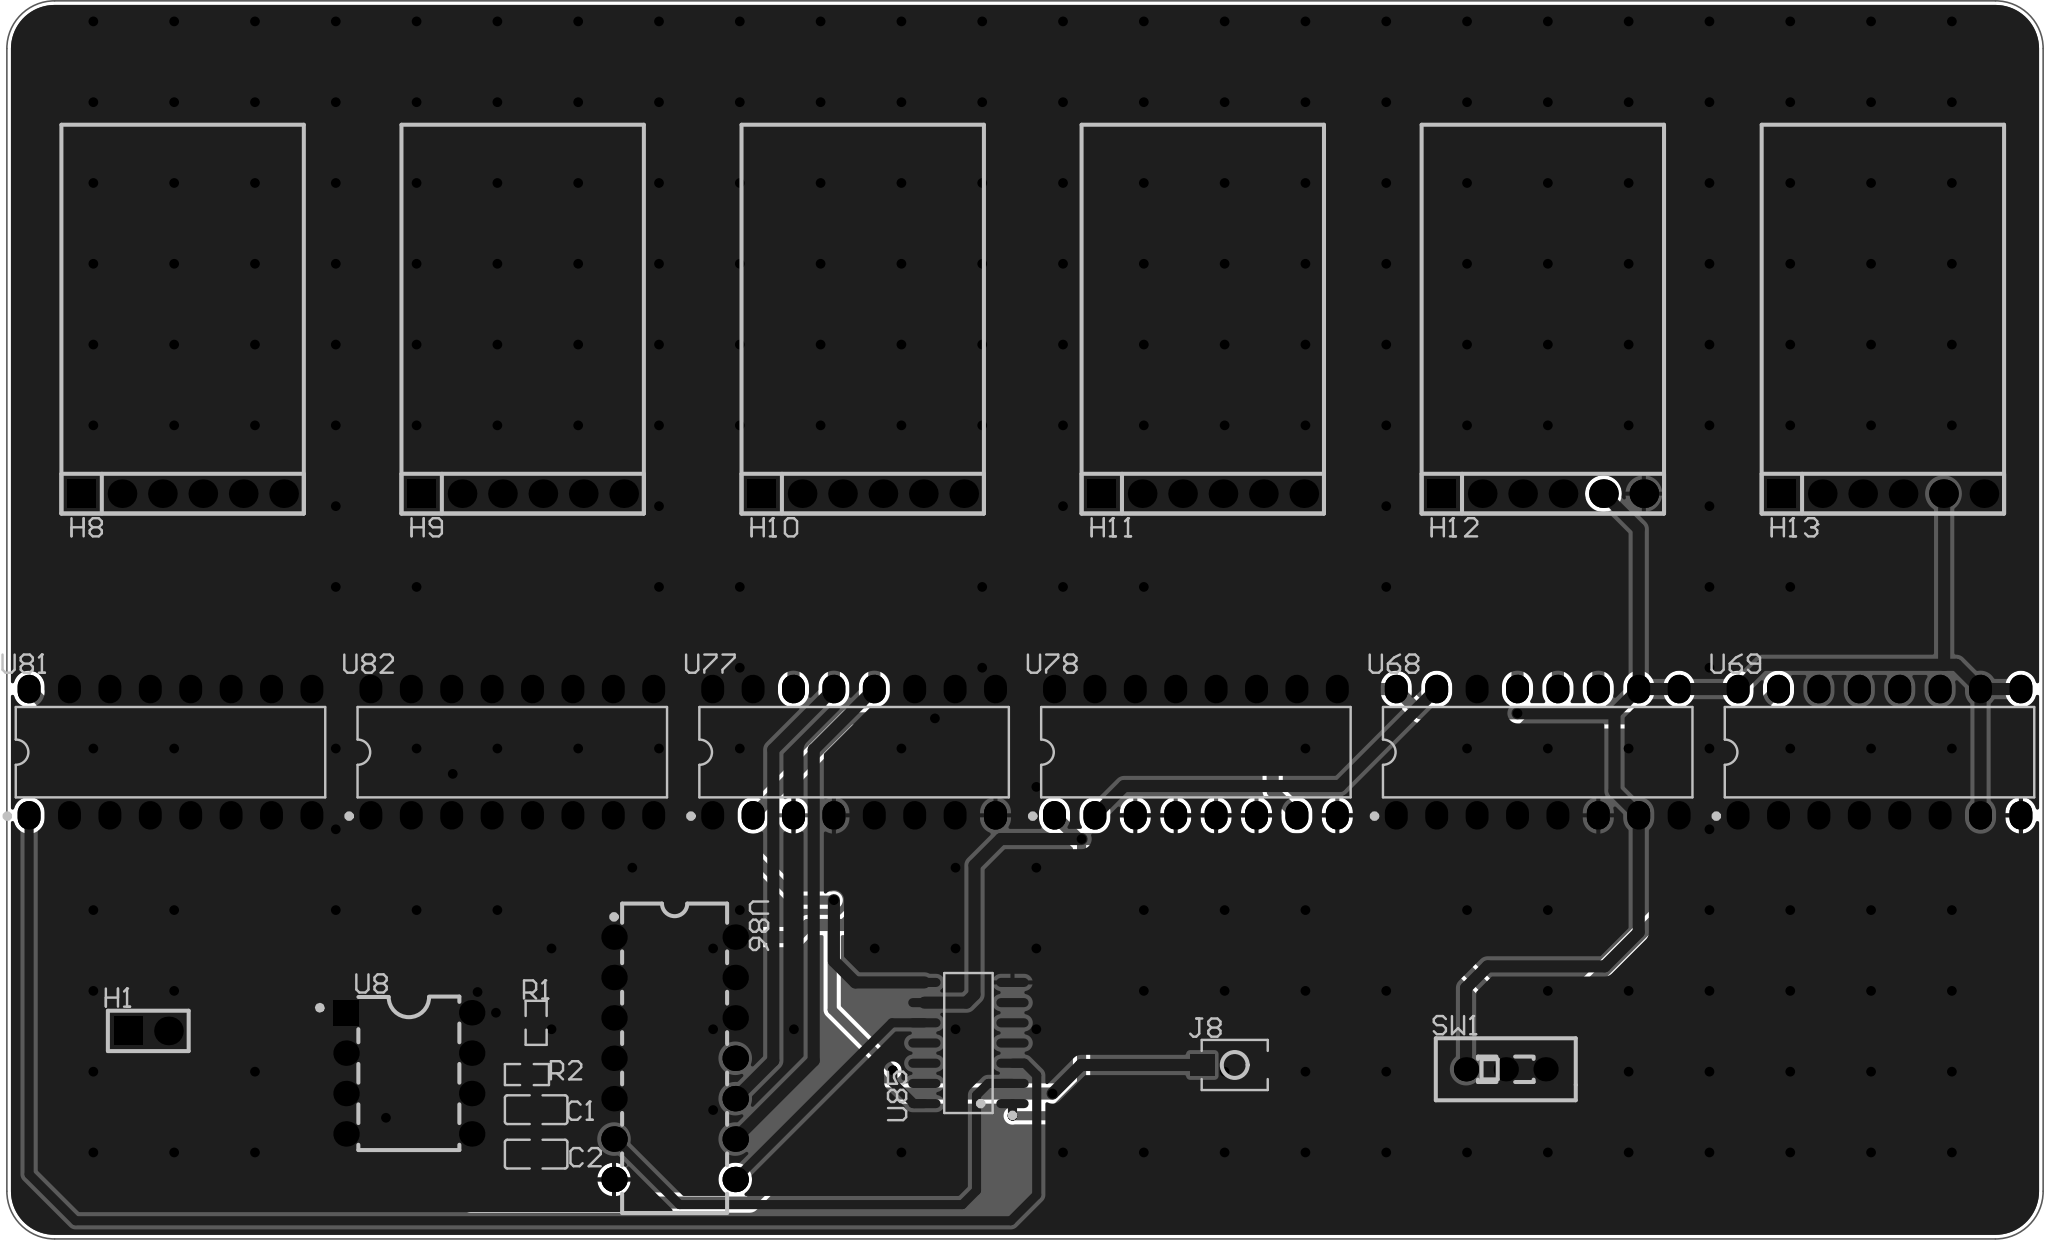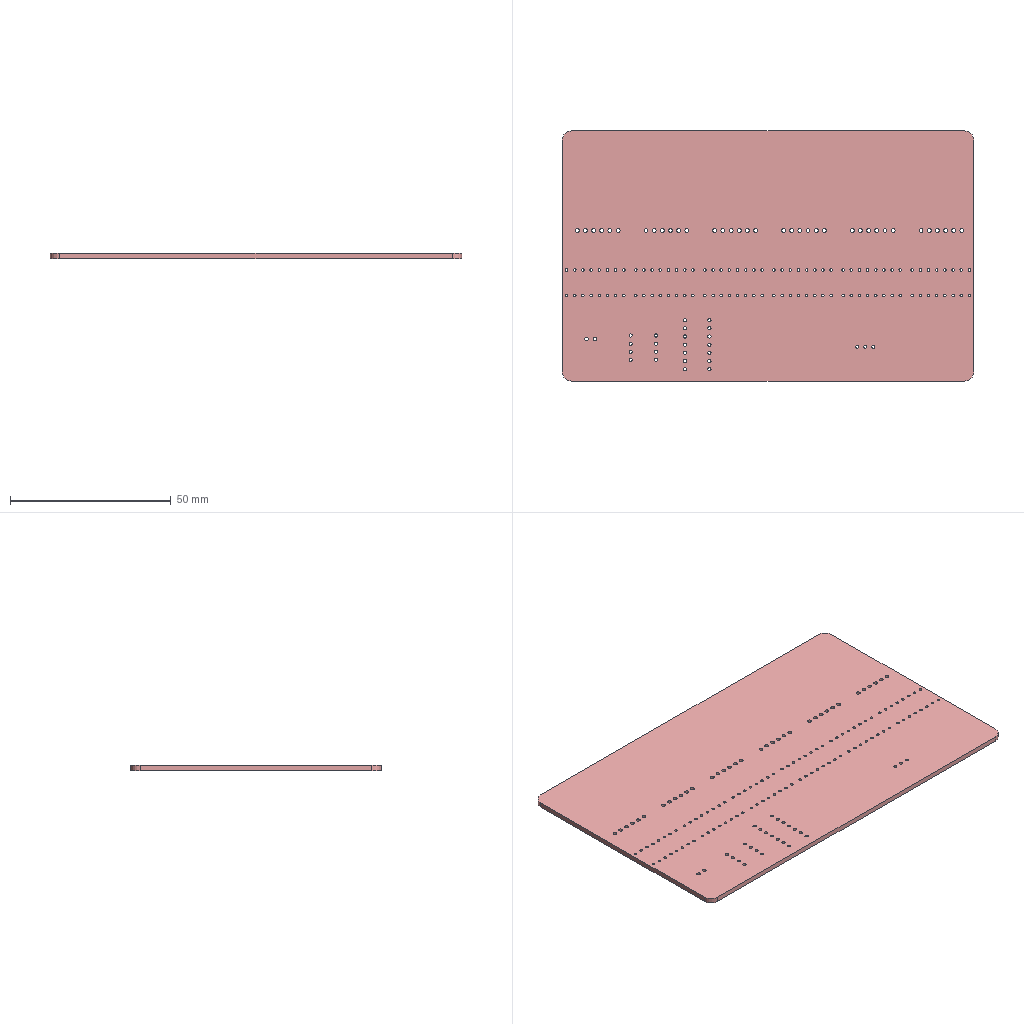Circuit board layout | Altium Designer | box 128 x 77.9 x 1.6 mm
Layer stack:
# Altium Designer layer stack of  (unit mm; dielectric type: 0 none, 1 core, 2 prepreg, 3 surface material)
index,name,kind,layer,copper_thickness_mm,dielectric_type,dielectric_thickness_mm,dielectric_material,dielectric_constant
0,Top Paste Mask Layer,other,,,,,,
1,Top Silkscreen Layer,other,,,,,,
2,Top Solder Mask Layer,dielectric,,,3,0.01,,3.3
3,Top Layer,copper,Top Layer,0.035,,,,
4,Dielectric1,dielectric,,,3,1.51,FR4,4.5
5,Bottom Layer,copper,Bottom Layer,0.035,,,,
6,Bottom Solder Mask Layer,dielectric,,,3,0.01,,3.3
7,Bottom Silkscreen Layer,other,,,,,,
8,Bottom Paste Mask Layer,other,,,,,,
# drill layer pairs: low layer,high layer
drill_pair,Top Layer,Bottom Layer
Part placement:
Designator,Comment,Layer,Footprint,Center-X(mm),Center-Y(mm),Rotation
H8,,TopLayer,HDR-TH_6P-P2.54-V-M-1,95.123,131.191,0
H9,,TopLayer,HDR-TH_6P-P2.54-V-M-1,116.501,131.191,0
H10,,TopLayer,HDR-TH_6P-P2.54-V-M-1,137.88,131.191,0
H11,,TopLayer,HDR-TH_6P-P2.54-V-M-1,159.258,131.191,0
H12,,TopLayer,HDR-TH_6P-P2.54-V-M-1,180.636,131.191,0
H13,,TopLayer,HDR-TH_6P-P2.54-V-M-1,202.014,131.191,0
C1,1uF,TopLayer,C0805,117.348,92.456,180
C2,10nF,TopLayer,C0805,117.348,89.662,180
H1,,TopLayer,HDR-TH_2P-P2.54-V-M-1,92.964,97.409,0
J8,轻触按键3*4*H,TopLayer,SW-SMD_L4.0-W2.9-LS5.0,161.266,95.267,0
R1,10k,TopLayer,R0603,117.348,97.917,90
R2,2.2k,TopLayer,R0603,116.769,94.663,0
SW1,开关,TopLayer,SW-TH_SS-12D01-GX,178.308,94.996,0
U8,NE555PE4,TopLayer,PDIP-8_L9.6-W6.4-P2.54-LS7.9-BL-1,109.347,94.742,270
U68,74LS160D,TopLayer,PDIP-16_L19.3-W6.4-P2.54-LS7.94-BL,180.315,114.935,0
U69,74LS160D,TopLayer,PDIP-16_L19.3-W6.4-P2.54-LS7.94-BL,201.803,114.935,0
U77,74LS160D,TopLayer,PDIP-16_L19.3-W6.4-P2.54-LS7.94-BL,137.338,114.935,0
U78,74LS160D,TopLayer,PDIP-16_L19.3-W6.4-P2.54-LS7.94-BL,158.826,114.935,0
U81,74LS160D,TopLayer,PDIP-16_L19.3-W6.4-P2.54-LS7.94-BL,94.361,114.935,0
U82,74LS160D,TopLayer,PDIP-16_L19.3-W6.4-P2.54-LS7.94-BL,115.849,114.935,0
U85,SN74LS08DR(LX),TopLayer,SOIC-14_L8.7-W3.9-P1.27-LS6.0-BL,144.526,96.647,90
U86,SN74LS00N(LX),TopLayer,PDIP-14_L19.3-W6.4-P2.54-LS7.9-BL,126.054,95.688,270
Pad and via stacks:
# Altium Designer via and pad stacks of  (unit mm). Each distinct definition once, with the count of objects using it.
# via: kind,start_layer,end_layer,hole_mm,diameter_mm,mode(0 simple;1 top-mid-bottom;2 full stack),diameter_per_layer,count,example_net
# pad: kind,layer,hole_mm,hole_type(0 round;1 square;2 slot),plating,top_size,top_shape(1 round;2 rect;3 octagon;9 rounded rect),mid_size,bottom_size,mode,footprint,size_per_layer,count,example
pad,Multi-Layer,1.2,0,plated,1.8x1.8,1,1.8x1.8,1.8x1.8,0,HDR-TH_6P-P2.54-V-M-1,,30,H8.6
pad,Multi-Layer,1.2,0,plated,1.8x1.8,2,1.8x1.8,1.8x1.8,0,HDR-TH_6P-P2.54-V-M-1,,6,H8.1
pad,Multi-Layer,1.1,0,plated,1.8x1.8,1,1.8x1.8,1.8x1.8,0,HDR-TH_2P-P2.54-V-M-1,,1,H1.2
pad,Multi-Layer,1.1,0,plated,1.8x1.8,2,1.8x1.8,1.8x1.8,0,HDR-TH_2P-P2.54-V-M-1,,1,H1.1
pad,Multi-Layer,0.9144,0,plated,1.524x1.524,1,1.524x1.524,1.524x1.524,0,SW-TH_SS-12D01-GX,,3,SW1.1
pad,Multi-Layer,1,0,plated,1.6x1.6,1,1.6x1.6,1.6x1.6,0,PDIP-8_L9.6-W6.4-P2.54-LS7.9-BL-1,,7,U8.8
pad,Multi-Layer,1,0,plated,1.6x1.6,2,1.6x1.6,1.6x1.6,0,PDIP-8_L9.6-W6.4-P2.54-LS7.9-BL-1,,1,U8.1
pad,Multi-Layer,0.8,0,plated,1.44x1.8,1,1.44x1.8,1.44x1.8,0,PDIP-16_L19.3-W6.4-P2.54-LS7.94-BL,,96,U68.1
pad,Multi-Layer,1,0,plated,1.6x1.6,1,1.6x1.6,1.6x1.6,0,PDIP-14_L19.3-W6.4-P2.54-LS7.9-BL,,14,U86.9
pad,Top Layer,0,0,plated,1.41x1.35,2,1.41x1.35,1.41x1.35,0,C0805,,4,C1.2
pad,Top Layer,0,0,plated,1.53x1.36,2,1.53x1.36,1.53x1.36,0,SW-SMD_L4.0-W2.9-LS5.0,,2,J8.1
pad,Top Layer,0,0,plated,0.8065x0.864,2,0.8065x0.864,0.8065x0.864,0,R0603,,4,R1.2
pad,Top Layer,0,0,plated,0.574x2.038,1,0.574x2.038,0.574x2.038,0,SOIC-14_L8.7-W3.9-P1.27-LS6.0-BL,,14,U85.1
via,Top Layer,Bottom Layer,0.3048,0.61,0,,260,$1N58085
Copper pours:
name,layer,net,type(0 solid;1 hatched;2 none)
Top Layer-GND,Top Layer,GND,0
Bottom Layer-GND,Bottom Layer,GND,0
Design rules, without the lines most boards share:
# Altium Designer design rules of  (exported by Altium Designer, unit mm)
# columns: name | kind | enabled | priority | scope1 | scope2 | descriptor | typed fields (field=value)
copperThickness1oz_2 | 2 | enabled | 2 | All | All | Width Constraint (Min=5mil) (Max=100mil) (Preferred=30mil) (All) |
viaSize | 11 | enabled | 1 | All | All | Routing Via (MinHoleWidth=11.811mil) (MaxHoleWidth=248.032mil) (PreferredHoleWidth=12.008mil) (MinWidth=19.685mil) (MaxWidth=393.701mil) (PreferedWidth=24.016mil) (All) | via_min_hole=0.3 via_max_hole=6.3 via_preferred_diameter=0.61 via_preferred_hole=0.305
solderMaskExpansion | 13 | enabled | 2 | All | All | Solder Mask Expansion (Expansion =2.008mil) (All) | expansion=0.051